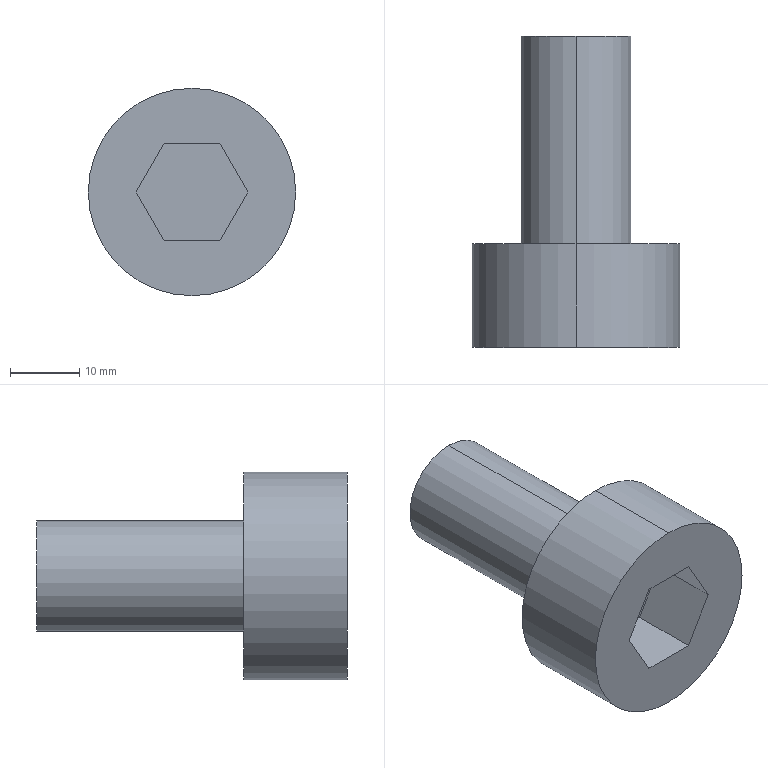Part | STEP file | M16X1.5 screw | 1 solid | 14 faces | box 30 x 45 x 30 mm | volume 14937 mm3 | plane 10 | cylinder 4 | commonest cylinder face diameters 16 x2 30 x2
STEP:
#1=CARTESIAN_POINT('',(0.,0.,0.));
#2=DIRECTION('',(0.,0.,1.));
#3=DIRECTION('',(1.,0.,0.));
#4=AXIS2_PLACEMENT_3D('',#1,#2,#3);
#5=CARTESIAN_POINT('',(0.,45.,-8.));
#6=VERTEX_POINT('',#5);
#7=CARTESIAN_POINT('',(0.,45.,8.));
#8=VERTEX_POINT('',#7);
#9=CARTESIAN_POINT('',(0.,45.,0.));
#10=DIRECTION('',(0.,-1.,0.));
#11=DIRECTION('',(0.,0.,-1.));
#12=AXIS2_PLACEMENT_3D('',#9,#10,#11);
#13=CIRCLE('',#12,8.);
#14=CARTESIAN_POINT('',(0.,0.,0.));
#15=DIRECTION('',(0.,-1.,0.));
#16=DIRECTION('',(0.,0.,-1.));
#17=AXIS2_PLACEMENT_3D('',#14,#15,#16);
#18=CYLINDRICAL_SURFACE('',#17,8.);
#19=CARTESIAN_POINT('',(0.,-45.));
#20=DIRECTION('',(1.,0.));
#21=VECTOR('',#20,1.);
#22=LINE('',#19,#21);
#23=(GEOMETRIC_REPRESENTATION_CONTEXT(2)PARAMETRIC_REPRESENTATION_CONTEXT()REPRESENTATION_CONTEXT('',''));
#24=DEFINITIONAL_REPRESENTATION('',(#22),#23);
#25=PCURVE('',#18,#24);
#26=CARTESIAN_POINT('',(8.,45.,0.));
#27=DIRECTION('',(0.,1.,0.));
#28=DIRECTION('',(0.,0.,1.));
#29=AXIS2_PLACEMENT_3D('',#26,#27,#28);
#30=PLANE('',#29);
#31=CARTESIAN_POINT('',(-8.,-8.));
#32=CARTESIAN_POINT('',(-8.,5.856));
#33=CARTESIAN_POINT('',(4.,-1.072));
#34=CARTESIAN_POINT('',(16.,-8.));
#35=CARTESIAN_POINT('',(4.,-14.928));
#36=CARTESIAN_POINT('',(-8.,-21.856));
#37=CARTESIAN_POINT('',(-8.,-8.));
#38=(BOUNDED_CURVE()B_SPLINE_CURVE(2,(#31,#32,#33,#34,#35,#36,#37),.UNSPECIFIED.,.T.,.F.)B_SPLINE_CURVE_WITH_KNOTS((1,2,2,2,2,1),(-2.094,0.,2.094,4.189,6.283,8.378),.UNSPECIFIED.)CURVE()GEOMETRIC_REPRESENTATION_ITEM()RATIONAL_B_SPLINE_CURVE((1.,0.5,1.,0.5,1.,0.5,1.))REPRESENTATION_ITEM(''));
#39=(GEOMETRIC_REPRESENTATION_CONTEXT(2)PARAMETRIC_REPRESENTATION_CONTEXT()REPRESENTATION_CONTEXT('',''));
#40=DEFINITIONAL_REPRESENTATION('',(#38),#39);
#41=PCURVE('',#30,#40);
#42=SURFACE_CURVE('',#13,(#25,#41),.PCURVE_S1.);
#43=EDGE_CURVE('',#6,#8,#42,.T.);
#44=ORIENTED_EDGE('',*,*,#43,.T.);
#45=CARTESIAN_POINT('',(0.,15.,8.));
#46=VERTEX_POINT('',#45);
#47=CARTESIAN_POINT('',(0.,0.,8.));
#48=DIRECTION('',(0.,-1.,0.));
#49=VECTOR('',#48,1.);
#50=LINE('',#47,#49);
#51=CARTESIAN_POINT('',(3.142,0.));
#52=DIRECTION('',(0.,1.));
#53=VECTOR('',#52,1.);
#54=LINE('',#51,#53);
#55=(GEOMETRIC_REPRESENTATION_CONTEXT(2)PARAMETRIC_REPRESENTATION_CONTEXT()REPRESENTATION_CONTEXT('',''));
#56=DEFINITIONAL_REPRESENTATION('',(#54),#55);
#57=PCURVE('',#18,#56);
#58=CARTESIAN_POINT('',(0.,0.,0.));
#59=DIRECTION('',(0.,-1.,0.));
#60=DIRECTION('',(0.,0.,-1.));
#61=AXIS2_PLACEMENT_3D('',#58,#59,#60);
#62=CYLINDRICAL_SURFACE('',#61,8.);
#63=CARTESIAN_POINT('',(3.142,0.));
#64=DIRECTION('',(0.,1.));
#65=VECTOR('',#64,1.);
#66=LINE('',#63,#65);
#67=(GEOMETRIC_REPRESENTATION_CONTEXT(2)PARAMETRIC_REPRESENTATION_CONTEXT()REPRESENTATION_CONTEXT('',''));
#68=DEFINITIONAL_REPRESENTATION('',(#66),#67);
#69=PCURVE('',#62,#68);
#70=SURFACE_CURVE('',#50,(#57,#69),.PCURVE_S1.);
#71=EDGE_CURVE('',#8,#46,#70,.T.);
#72=ORIENTED_EDGE('',*,*,#71,.T.);
#73=CARTESIAN_POINT('',(0.,15.,-8.));
#74=VERTEX_POINT('',#73);
#75=CARTESIAN_POINT('',(0.,15.,0.));
#76=DIRECTION('',(0.,-1.,0.));
#77=DIRECTION('',(0.,0.,-1.));
#78=AXIS2_PLACEMENT_3D('',#75,#76,#77);
#79=CIRCLE('',#78,8.);
#80=CARTESIAN_POINT('',(0.,-15.));
#81=DIRECTION('',(1.,0.));
#82=VECTOR('',#81,1.);
#83=LINE('',#80,#82);
#84=(GEOMETRIC_REPRESENTATION_CONTEXT(2)PARAMETRIC_REPRESENTATION_CONTEXT()REPRESENTATION_CONTEXT('',''));
#85=DEFINITIONAL_REPRESENTATION('',(#83),#84);
#86=PCURVE('',#18,#85);
#87=CARTESIAN_POINT('',(15.,15.,0.));
#88=DIRECTION('',(0.,1.,0.));
#89=DIRECTION('',(0.,0.,1.));
#90=AXIS2_PLACEMENT_3D('',#87,#88,#89);
#91=PLANE('',#90);
#92=CARTESIAN_POINT('',(-8.,-15.));
#93=CARTESIAN_POINT('',(-8.,-1.144));
#94=CARTESIAN_POINT('',(4.,-8.072));
#95=CARTESIAN_POINT('',(16.,-15.));
#96=CARTESIAN_POINT('',(4.,-21.928));
#97=CARTESIAN_POINT('',(-8.,-28.856));
#98=CARTESIAN_POINT('',(-8.,-15.));
#99=(BOUNDED_CURVE()B_SPLINE_CURVE(2,(#92,#93,#94,#95,#96,#97,#98),.UNSPECIFIED.,.T.,.F.)B_SPLINE_CURVE_WITH_KNOTS((1,2,2,2,2,1),(-2.094,0.,2.094,4.189,6.283,8.378),.UNSPECIFIED.)CURVE()GEOMETRIC_REPRESENTATION_ITEM()RATIONAL_B_SPLINE_CURVE((1.,0.5,1.,0.5,1.,0.5,1.))REPRESENTATION_ITEM(''));
#100=(GEOMETRIC_REPRESENTATION_CONTEXT(2)PARAMETRIC_REPRESENTATION_CONTEXT()REPRESENTATION_CONTEXT('',''));
#101=DEFINITIONAL_REPRESENTATION('',(#99),#100);
#102=PCURVE('',#91,#101);
#103=SURFACE_CURVE('',#79,(#86,#102),.PCURVE_S1.);
#104=EDGE_CURVE('',#74,#46,#103,.T.);
#105=ORIENTED_EDGE('',*,*,#104,.F.);
#106=CARTESIAN_POINT('',(0.,0.,-8.));
#107=DIRECTION('',(0.,-1.,0.));
#108=VECTOR('',#107,1.);
#109=LINE('',#106,#108);
#110=CARTESIAN_POINT('',(0.,0.));
#111=DIRECTION('',(0.,1.));
#112=VECTOR('',#111,1.);
#113=LINE('',#110,#112);
#114=(GEOMETRIC_REPRESENTATION_CONTEXT(2)PARAMETRIC_REPRESENTATION_CONTEXT()REPRESENTATION_CONTEXT('',''));
#115=DEFINITIONAL_REPRESENTATION('',(#113),#114);
#116=PCURVE('',#18,#115);
#117=CARTESIAN_POINT('',(6.283,0.));
#118=DIRECTION('',(0.,1.));
#119=VECTOR('',#118,1.);
#120=LINE('',#117,#119);
#121=(GEOMETRIC_REPRESENTATION_CONTEXT(2)PARAMETRIC_REPRESENTATION_CONTEXT()REPRESENTATION_CONTEXT('',''));
#122=DEFINITIONAL_REPRESENTATION('',(#120),#121);
#123=PCURVE('',#62,#122);
#124=SURFACE_CURVE('',#109,(#116,#123),.PCURVE_S1.);
#125=EDGE_CURVE('',#6,#74,#124,.T.);
#126=ORIENTED_EDGE('',*,*,#125,.F.);
#127=EDGE_LOOP('',(#44,#72,#105,#126));
#128=FACE_BOUND('',#127,.T.);
#129=ADVANCED_FACE('',(#128),#18,.T.);
#130=CARTESIAN_POINT('',(0.,15.,-15.));
#131=VERTEX_POINT('',#130);
#132=CARTESIAN_POINT('',(0.,15.,15.));
#133=VERTEX_POINT('',#132);
#134=CARTESIAN_POINT('',(0.,15.,0.));
#135=DIRECTION('',(0.,-1.,0.));
#136=DIRECTION('',(0.,0.,-1.));
#137=AXIS2_PLACEMENT_3D('',#134,#135,#136);
#138=CIRCLE('',#137,15.);
#139=CARTESIAN_POINT('',(0.,0.,0.));
#140=DIRECTION('',(0.,-1.,0.));
#141=DIRECTION('',(0.,0.,-1.));
#142=AXIS2_PLACEMENT_3D('',#139,#140,#141);
#143=CYLINDRICAL_SURFACE('',#142,15.);
#144=CARTESIAN_POINT('',(0.,-15.));
#145=DIRECTION('',(1.,0.));
#146=VECTOR('',#145,1.);
#147=LINE('',#144,#146);
#148=(GEOMETRIC_REPRESENTATION_CONTEXT(2)PARAMETRIC_REPRESENTATION_CONTEXT()REPRESENTATION_CONTEXT('',''));
#149=DEFINITIONAL_REPRESENTATION('',(#147),#148);
#150=PCURVE('',#143,#149);
#151=CARTESIAN_POINT('',(-15.,-15.));
#152=CARTESIAN_POINT('',(-15.,10.981));
#153=CARTESIAN_POINT('',(7.5,-2.01));
#154=CARTESIAN_POINT('',(30.,-15.));
#155=CARTESIAN_POINT('',(7.5,-27.99));
#156=CARTESIAN_POINT('',(-15.,-40.981));
#157=CARTESIAN_POINT('',(-15.,-15.));
#158=(BOUNDED_CURVE()B_SPLINE_CURVE(2,(#151,#152,#153,#154,#155,#156,#157),.UNSPECIFIED.,.T.,.F.)B_SPLINE_CURVE_WITH_KNOTS((1,2,2,2,2,1),(-2.094,0.,2.094,4.189,6.283,8.378),.UNSPECIFIED.)CURVE()GEOMETRIC_REPRESENTATION_ITEM()RATIONAL_B_SPLINE_CURVE((1.,0.5,1.,0.5,1.,0.5,1.))REPRESENTATION_ITEM(''));
#159=(GEOMETRIC_REPRESENTATION_CONTEXT(2)PARAMETRIC_REPRESENTATION_CONTEXT()REPRESENTATION_CONTEXT('',''));
#160=DEFINITIONAL_REPRESENTATION('',(#158),#159);
#161=PCURVE('',#91,#160);
#162=SURFACE_CURVE('',#138,(#150,#161),.PCURVE_S1.);
#163=EDGE_CURVE('',#131,#133,#162,.T.);
#164=ORIENTED_EDGE('',*,*,#163,.T.);
#165=CARTESIAN_POINT('',(0.,0.,15.));
#166=VERTEX_POINT('',#165);
#167=CARTESIAN_POINT('',(0.,0.,15.));
#168=DIRECTION('',(0.,-1.,0.));
#169=VECTOR('',#168,1.);
#170=LINE('',#167,#169);
#171=CARTESIAN_POINT('',(3.142,0.));
#172=DIRECTION('',(0.,1.));
#173=VECTOR('',#172,1.);
#174=LINE('',#171,#173);
#175=(GEOMETRIC_REPRESENTATION_CONTEXT(2)PARAMETRIC_REPRESENTATION_CONTEXT()REPRESENTATION_CONTEXT('',''));
#176=DEFINITIONAL_REPRESENTATION('',(#174),#175);
#177=PCURVE('',#143,#176);
#178=CARTESIAN_POINT('',(0.,0.,0.));
#179=DIRECTION('',(0.,-1.,0.));
#180=DIRECTION('',(0.,0.,-1.));
#181=AXIS2_PLACEMENT_3D('',#178,#179,#180);
#182=CYLINDRICAL_SURFACE('',#181,15.);
#183=CARTESIAN_POINT('',(3.142,0.));
#184=DIRECTION('',(0.,1.));
#185=VECTOR('',#184,1.);
#186=LINE('',#183,#185);
#187=(GEOMETRIC_REPRESENTATION_CONTEXT(2)PARAMETRIC_REPRESENTATION_CONTEXT()REPRESENTATION_CONTEXT('',''));
#188=DEFINITIONAL_REPRESENTATION('',(#186),#187);
#189=PCURVE('',#182,#188);
#190=SURFACE_CURVE('',#170,(#177,#189),.PCURVE_S1.);
#191=EDGE_CURVE('',#133,#166,#190,.T.);
#192=ORIENTED_EDGE('',*,*,#191,.T.);
#193=CARTESIAN_POINT('',(0.,0.,-15.));
#194=VERTEX_POINT('',#193);
#195=CARTESIAN_POINT('',(0.,0.,0.));
#196=DIRECTION('',(0.,-1.,0.));
#197=DIRECTION('',(0.,0.,-1.));
#198=AXIS2_PLACEMENT_3D('',#195,#196,#197);
#199=CIRCLE('',#198,15.);
#200=CARTESIAN_POINT('',(0.,0.));
#201=DIRECTION('',(1.,0.));
#202=VECTOR('',#201,1.);
#203=LINE('',#200,#202);
#204=(GEOMETRIC_REPRESENTATION_CONTEXT(2)PARAMETRIC_REPRESENTATION_CONTEXT()REPRESENTATION_CONTEXT('',''));
#205=DEFINITIONAL_REPRESENTATION('',(#203),#204);
#206=PCURVE('',#143,#205);
#207=CARTESIAN_POINT('',(0.,0.,0.));
#208=DIRECTION('',(0.,-1.,0.));
#209=DIRECTION('',(0.,0.,-1.));
#210=AXIS2_PLACEMENT_3D('',#207,#208,#209);
#211=PLANE('',#210);
#212=CARTESIAN_POINT('',(0.,0.));
#213=DIRECTION('',(1.,0.));
#214=AXIS2_PLACEMENT_2D('',#212,#213);
#215=CIRCLE('',#214,15.);
#216=(GEOMETRIC_REPRESENTATION_CONTEXT(2)PARAMETRIC_REPRESENTATION_CONTEXT()REPRESENTATION_CONTEXT('',''));
#217=DEFINITIONAL_REPRESENTATION('',(#215),#216);
#218=PCURVE('',#211,#217);
#219=SURFACE_CURVE('',#199,(#206,#218),.PCURVE_S1.);
#220=EDGE_CURVE('',#194,#166,#219,.T.);
#221=ORIENTED_EDGE('',*,*,#220,.F.);
#222=CARTESIAN_POINT('',(0.,0.,-15.));
#223=DIRECTION('',(0.,-1.,0.));
#224=VECTOR('',#223,1.);
#225=LINE('',#222,#224);
#226=CARTESIAN_POINT('',(0.,0.));
#227=DIRECTION('',(0.,1.));
#228=VECTOR('',#227,1.);
#229=LINE('',#226,#228);
#230=(GEOMETRIC_REPRESENTATION_CONTEXT(2)PARAMETRIC_REPRESENTATION_CONTEXT()REPRESENTATION_CONTEXT('',''));
#231=DEFINITIONAL_REPRESENTATION('',(#229),#230);
#232=PCURVE('',#143,#231);
#233=CARTESIAN_POINT('',(6.283,0.));
#234=DIRECTION('',(0.,1.));
#235=VECTOR('',#234,1.);
#236=LINE('',#233,#235);
#237=(GEOMETRIC_REPRESENTATION_CONTEXT(2)PARAMETRIC_REPRESENTATION_CONTEXT()REPRESENTATION_CONTEXT('',''));
#238=DEFINITIONAL_REPRESENTATION('',(#236),#237);
#239=PCURVE('',#182,#238);
#240=SURFACE_CURVE('',#225,(#232,#239),.PCURVE_S1.);
#241=EDGE_CURVE('',#131,#194,#240,.T.);
#242=ORIENTED_EDGE('',*,*,#241,.F.);
#243=EDGE_LOOP('',(#164,#192,#221,#242));
#244=FACE_BOUND('',#243,.T.);
#245=ADVANCED_FACE('',(#244),#143,.T.);
#246=CARTESIAN_POINT('',(-4.041,0.,7.));
#247=VERTEX_POINT('',#246);
#248=CARTESIAN_POINT('',(-8.083,0.,0.));
#249=VERTEX_POINT('',#248);
#250=CARTESIAN_POINT('',(-4.041,0.,7.));
#251=DIRECTION('',(-0.5,0.,-0.866));
#252=VECTOR('',#251,1.);
#253=LINE('',#250,#252);
#254=CARTESIAN_POINT('',(-7.,-4.041));
#255=DIRECTION('',(0.866,-0.5));
#256=VECTOR('',#255,1.);
#257=LINE('',#254,#256);
#258=(GEOMETRIC_REPRESENTATION_CONTEXT(2)PARAMETRIC_REPRESENTATION_CONTEXT()REPRESENTATION_CONTEXT('',''));
#259=DEFINITIONAL_REPRESENTATION('',(#257),#258);
#260=PCURVE('',#211,#259);
#261=CARTESIAN_POINT('',(-4.041,10.,7.));
#262=DIRECTION('',(-0.866,0.,0.5));
#263=DIRECTION('',(0.5,0.,0.866));
#264=AXIS2_PLACEMENT_3D('',#261,#262,#263);
#265=PLANE('',#264);
#266=CARTESIAN_POINT('',(0.,-10.));
#267=DIRECTION('',(-1.,0.));
#268=VECTOR('',#267,1.);
#269=LINE('',#266,#268);
#270=(GEOMETRIC_REPRESENTATION_CONTEXT(2)PARAMETRIC_REPRESENTATION_CONTEXT()REPRESENTATION_CONTEXT('',''));
#271=DEFINITIONAL_REPRESENTATION('',(#269),#270);
#272=PCURVE('',#265,#271);
#273=SURFACE_CURVE('',#253,(#260,#272),.PCURVE_S1.);
#274=EDGE_CURVE('',#247,#249,#273,.T.);
#275=ORIENTED_EDGE('',*,*,#274,.F.);
#276=CARTESIAN_POINT('',(4.041,0.,7.));
#277=VERTEX_POINT('',#276);
#278=CARTESIAN_POINT('',(4.041,0.,7.));
#279=DIRECTION('',(-1.,0.,0.));
#280=VECTOR('',#279,1.);
#281=LINE('',#278,#280);
#282=CARTESIAN_POINT('',(-7.,4.041));
#283=DIRECTION('',(0.,-1.));
#284=VECTOR('',#283,1.);
#285=LINE('',#282,#284);
#286=(GEOMETRIC_REPRESENTATION_CONTEXT(2)PARAMETRIC_REPRESENTATION_CONTEXT()REPRESENTATION_CONTEXT('',''));
#287=DEFINITIONAL_REPRESENTATION('',(#285),#286);
#288=PCURVE('',#211,#287);
#289=CARTESIAN_POINT('',(4.041,10.,7.));
#290=DIRECTION('',(0.,0.,1.));
#291=DIRECTION('',(1.,0.,0.));
#292=AXIS2_PLACEMENT_3D('',#289,#290,#291);
#293=PLANE('',#292);
#294=CARTESIAN_POINT('',(0.,-10.));
#295=DIRECTION('',(-1.,0.));
#296=VECTOR('',#295,1.);
#297=LINE('',#294,#296);
#298=(GEOMETRIC_REPRESENTATION_CONTEXT(2)PARAMETRIC_REPRESENTATION_CONTEXT()REPRESENTATION_CONTEXT('',''));
#299=DEFINITIONAL_REPRESENTATION('',(#297),#298);
#300=PCURVE('',#293,#299);
#301=SURFACE_CURVE('',#281,(#288,#300),.PCURVE_S1.);
#302=EDGE_CURVE('',#277,#247,#301,.T.);
#303=ORIENTED_EDGE('',*,*,#302,.F.);
#304=CARTESIAN_POINT('',(8.083,0.,0.));
#305=VERTEX_POINT('',#304);
#306=CARTESIAN_POINT('',(8.083,0.,0.));
#307=DIRECTION('',(-0.5,0.,0.866));
#308=VECTOR('',#307,1.);
#309=LINE('',#306,#308);
#310=CARTESIAN_POINT('',(0.,8.083));
#311=DIRECTION('',(-0.866,-0.5));
#312=VECTOR('',#311,1.);
#313=LINE('',#310,#312);
#314=(GEOMETRIC_REPRESENTATION_CONTEXT(2)PARAMETRIC_REPRESENTATION_CONTEXT()REPRESENTATION_CONTEXT('',''));
#315=DEFINITIONAL_REPRESENTATION('',(#313),#314);
#316=PCURVE('',#211,#315);
#317=CARTESIAN_POINT('',(8.083,10.,0.));
#318=DIRECTION('',(0.866,0.,0.5));
#319=DIRECTION('',(0.5,0.,-0.866));
#320=AXIS2_PLACEMENT_3D('',#317,#318,#319);
#321=PLANE('',#320);
#322=CARTESIAN_POINT('',(0.,-10.));
#323=DIRECTION('',(-1.,0.));
#324=VECTOR('',#323,1.);
#325=LINE('',#322,#324);
#326=(GEOMETRIC_REPRESENTATION_CONTEXT(2)PARAMETRIC_REPRESENTATION_CONTEXT()REPRESENTATION_CONTEXT('',''));
#327=DEFINITIONAL_REPRESENTATION('',(#325),#326);
#328=PCURVE('',#321,#327);
#329=SURFACE_CURVE('',#309,(#316,#328),.PCURVE_S1.);
#330=EDGE_CURVE('',#305,#277,#329,.T.);
#331=ORIENTED_EDGE('',*,*,#330,.F.);
#332=CARTESIAN_POINT('',(4.041,0.,-7.));
#333=VERTEX_POINT('',#332);
#334=CARTESIAN_POINT('',(4.041,0.,-7.));
#335=DIRECTION('',(0.5,0.,0.866));
#336=VECTOR('',#335,1.);
#337=LINE('',#334,#336);
#338=CARTESIAN_POINT('',(7.,4.041));
#339=DIRECTION('',(-0.866,0.5));
#340=VECTOR('',#339,1.);
#341=LINE('',#338,#340);
#342=(GEOMETRIC_REPRESENTATION_CONTEXT(2)PARAMETRIC_REPRESENTATION_CONTEXT()REPRESENTATION_CONTEXT('',''));
#343=DEFINITIONAL_REPRESENTATION('',(#341),#342);
#344=PCURVE('',#211,#343);
#345=CARTESIAN_POINT('',(4.041,10.,-7.));
#346=DIRECTION('',(0.866,0.,-0.5));
#347=DIRECTION('',(-0.5,0.,-0.866));
#348=AXIS2_PLACEMENT_3D('',#345,#346,#347);
#349=PLANE('',#348);
#350=CARTESIAN_POINT('',(0.,-10.));
#351=DIRECTION('',(-1.,0.));
#352=VECTOR('',#351,1.);
#353=LINE('',#350,#352);
#354=(GEOMETRIC_REPRESENTATION_CONTEXT(2)PARAMETRIC_REPRESENTATION_CONTEXT()REPRESENTATION_CONTEXT('',''));
#355=DEFINITIONAL_REPRESENTATION('',(#353),#354);
#356=PCURVE('',#349,#355);
#357=SURFACE_CURVE('',#337,(#344,#356),.PCURVE_S1.);
#358=EDGE_CURVE('',#333,#305,#357,.T.);
#359=ORIENTED_EDGE('',*,*,#358,.F.);
#360=CARTESIAN_POINT('',(-4.041,0.,-7.));
#361=VERTEX_POINT('',#360);
#362=CARTESIAN_POINT('',(-4.041,0.,-7.));
#363=DIRECTION('',(1.,0.,0.));
#364=VECTOR('',#363,1.);
#365=LINE('',#362,#364);
#366=CARTESIAN_POINT('',(7.,-4.041));
#367=DIRECTION('',(0.,1.));
#368=VECTOR('',#367,1.);
#369=LINE('',#366,#368);
#370=(GEOMETRIC_REPRESENTATION_CONTEXT(2)PARAMETRIC_REPRESENTATION_CONTEXT()REPRESENTATION_CONTEXT('',''));
#371=DEFINITIONAL_REPRESENTATION('',(#369),#370);
#372=PCURVE('',#211,#371);
#373=CARTESIAN_POINT('',(-4.041,10.,-7.));
#374=DIRECTION('',(0.,0.,-1.));
#375=DIRECTION('',(-1.,0.,0.));
#376=AXIS2_PLACEMENT_3D('',#373,#374,#375);
#377=PLANE('',#376);
#378=CARTESIAN_POINT('',(0.,-10.));
#379=DIRECTION('',(-1.,0.));
#380=VECTOR('',#379,1.);
#381=LINE('',#378,#380);
#382=(GEOMETRIC_REPRESENTATION_CONTEXT(2)PARAMETRIC_REPRESENTATION_CONTEXT()REPRESENTATION_CONTEXT('',''));
#383=DEFINITIONAL_REPRESENTATION('',(#381),#382);
#384=PCURVE('',#377,#383);
#385=SURFACE_CURVE('',#365,(#372,#384),.PCURVE_S1.);
#386=EDGE_CURVE('',#361,#333,#385,.T.);
#387=ORIENTED_EDGE('',*,*,#386,.F.);
#388=CARTESIAN_POINT('',(-8.083,0.,0.));
#389=DIRECTION('',(0.5,0.,-0.866));
#390=VECTOR('',#389,1.);
#391=LINE('',#388,#390);
#392=CARTESIAN_POINT('',(0.,-8.083));
#393=DIRECTION('',(0.866,0.5));
#394=VECTOR('',#393,1.);
#395=LINE('',#392,#394);
#396=(GEOMETRIC_REPRESENTATION_CONTEXT(2)PARAMETRIC_REPRESENTATION_CONTEXT()REPRESENTATION_CONTEXT('',''));
#397=DEFINITIONAL_REPRESENTATION('',(#395),#396);
#398=PCURVE('',#211,#397);
#399=CARTESIAN_POINT('',(-8.083,10.,0.));
#400=DIRECTION('',(-0.866,0.,-0.5));
#401=DIRECTION('',(-0.5,0.,0.866));
#402=AXIS2_PLACEMENT_3D('',#399,#400,#401);
#403=PLANE('',#402);
#404=CARTESIAN_POINT('',(0.,-10.));
#405=DIRECTION('',(-1.,0.));
#406=VECTOR('',#405,1.);
#407=LINE('',#404,#406);
#408=(GEOMETRIC_REPRESENTATION_CONTEXT(2)PARAMETRIC_REPRESENTATION_CONTEXT()REPRESENTATION_CONTEXT('',''));
#409=DEFINITIONAL_REPRESENTATION('',(#407),#408);
#410=PCURVE('',#403,#409);
#411=SURFACE_CURVE('',#391,(#398,#410),.PCURVE_S1.);
#412=EDGE_CURVE('',#249,#361,#411,.T.);
#413=ORIENTED_EDGE('',*,*,#412,.F.);
#414=EDGE_LOOP('',(#275,#303,#331,#359,#387,#413));
#415=FACE_BOUND('',#414,.T.);
#416=ORIENTED_EDGE('',*,*,#220,.T.);
#417=CARTESIAN_POINT('',(0.,0.,0.));
#418=DIRECTION('',(0.,-1.,0.));
#419=DIRECTION('',(0.,0.,-1.));
#420=AXIS2_PLACEMENT_3D('',#417,#418,#419);
#421=CIRCLE('',#420,15.);
#422=CARTESIAN_POINT('',(0.,0.));
#423=DIRECTION('',(1.,0.));
#424=AXIS2_PLACEMENT_2D('',#422,#423);
#425=CIRCLE('',#424,15.);
#426=(GEOMETRIC_REPRESENTATION_CONTEXT(2)PARAMETRIC_REPRESENTATION_CONTEXT()REPRESENTATION_CONTEXT('',''));
#427=DEFINITIONAL_REPRESENTATION('',(#425),#426);
#428=PCURVE('',#211,#427);
#429=CARTESIAN_POINT('',(0.,0.));
#430=DIRECTION('',(1.,0.));
#431=VECTOR('',#430,1.);
#432=LINE('',#429,#431);
#433=(GEOMETRIC_REPRESENTATION_CONTEXT(2)PARAMETRIC_REPRESENTATION_CONTEXT()REPRESENTATION_CONTEXT('',''));
#434=DEFINITIONAL_REPRESENTATION('',(#432),#433);
#435=PCURVE('',#182,#434);
#436=SURFACE_CURVE('',#421,(#428,#435),.PCURVE_S1.);
#437=EDGE_CURVE('',#166,#194,#436,.T.);
#438=ORIENTED_EDGE('',*,*,#437,.T.);
#439=EDGE_LOOP('',(#416,#438));
#440=FACE_BOUND('',#439,.T.);
#441=ADVANCED_FACE('',(#415,#440),#211,.T.);
#442=ORIENTED_EDGE('',*,*,#191,.F.);
#443=CARTESIAN_POINT('',(0.,15.,0.));
#444=DIRECTION('',(0.,-1.,0.));
#445=DIRECTION('',(0.,0.,-1.));
#446=AXIS2_PLACEMENT_3D('',#443,#444,#445);
#447=CIRCLE('',#446,15.);
#448=CARTESIAN_POINT('',(0.,-15.));
#449=DIRECTION('',(1.,0.));
#450=VECTOR('',#449,1.);
#451=LINE('',#448,#450);
#452=(GEOMETRIC_REPRESENTATION_CONTEXT(2)PARAMETRIC_REPRESENTATION_CONTEXT()REPRESENTATION_CONTEXT('',''));
#453=DEFINITIONAL_REPRESENTATION('',(#451),#452);
#454=PCURVE('',#182,#453);
#455=CARTESIAN_POINT('',(-15.,-15.));
#456=CARTESIAN_POINT('',(-15.,10.981));
#457=CARTESIAN_POINT('',(7.5,-2.01));
#458=CARTESIAN_POINT('',(30.,-15.));
#459=CARTESIAN_POINT('',(7.5,-27.99));
#460=CARTESIAN_POINT('',(-15.,-40.981));
#461=CARTESIAN_POINT('',(-15.,-15.));
#462=(BOUNDED_CURVE()B_SPLINE_CURVE(2,(#455,#456,#457,#458,#459,#460,#461),.UNSPECIFIED.,.T.,.F.)B_SPLINE_CURVE_WITH_KNOTS((1,2,2,2,2,1),(-2.094,0.,2.094,4.189,6.283,8.378),.UNSPECIFIED.)CURVE()GEOMETRIC_REPRESENTATION_ITEM()RATIONAL_B_SPLINE_CURVE((1.,0.5,1.,0.5,1.,0.5,1.))REPRESENTATION_ITEM(''));
#463=(GEOMETRIC_REPRESENTATION_CONTEXT(2)PARAMETRIC_REPRESENTATION_CONTEXT()REPRESENTATION_CONTEXT('',''));
#464=DEFINITIONAL_REPRESENTATION('',(#462),#463);
#465=PCURVE('',#91,#464);
#466=SURFACE_CURVE('',#447,(#454,#465),.PCURVE_S1.);
#467=EDGE_CURVE('',#133,#131,#466,.T.);
#468=ORIENTED_EDGE('',*,*,#467,.T.);
#469=ORIENTED_EDGE('',*,*,#241,.T.);
#470=ORIENTED_EDGE('',*,*,#437,.F.);
#471=EDGE_LOOP('',(#442,#468,#469,#470));
#472=FACE_BOUND('',#471,.T.);
#473=ADVANCED_FACE('',(#472),#182,.T.);
#474=ORIENTED_EDGE('',*,*,#104,.T.);
#475=CARTESIAN_POINT('',(0.,15.,0.));
#476=DIRECTION('',(0.,-1.,0.));
#477=DIRECTION('',(0.,0.,-1.));
#478=AXIS2_PLACEMENT_3D('',#475,#476,#477);
#479=CIRCLE('',#478,8.);
#480=CARTESIAN_POINT('',(-8.,-15.));
#481=CARTESIAN_POINT('',(-8.,-1.144));
#482=CARTESIAN_POINT('',(4.,-8.072));
#483=CARTESIAN_POINT('',(16.,-15.));
#484=CARTESIAN_POINT('',(4.,-21.928));
#485=CARTESIAN_POINT('',(-8.,-28.856));
#486=CARTESIAN_POINT('',(-8.,-15.));
#487=(BOUNDED_CURVE()B_SPLINE_CURVE(2,(#480,#481,#482,#483,#484,#485,#486),.UNSPECIFIED.,.T.,.F.)B_SPLINE_CURVE_WITH_KNOTS((1,2,2,2,2,1),(-2.094,0.,2.094,4.189,6.283,8.378),.UNSPECIFIED.)CURVE()GEOMETRIC_REPRESENTATION_ITEM()RATIONAL_B_SPLINE_CURVE((1.,0.5,1.,0.5,1.,0.5,1.))REPRESENTATION_ITEM(''));
#488=(GEOMETRIC_REPRESENTATION_CONTEXT(2)PARAMETRIC_REPRESENTATION_CONTEXT()REPRESENTATION_CONTEXT('',''));
#489=DEFINITIONAL_REPRESENTATION('',(#487),#488);
#490=PCURVE('',#91,#489);
#491=CARTESIAN_POINT('',(0.,-15.));
#492=DIRECTION('',(1.,0.));
#493=VECTOR('',#492,1.);
#494=LINE('',#491,#493);
#495=(GEOMETRIC_REPRESENTATION_CONTEXT(2)PARAMETRIC_REPRESENTATION_CONTEXT()REPRESENTATION_CONTEXT('',''));
#496=DEFINITIONAL_REPRESENTATION('',(#494),#495);
#497=PCURVE('',#62,#496);
#498=SURFACE_CURVE('',#479,(#490,#497),.PCURVE_S1.);
#499=EDGE_CURVE('',#46,#74,#498,.T.);
#500=ORIENTED_EDGE('',*,*,#499,.T.);
#501=EDGE_LOOP('',(#474,#500));
#502=FACE_BOUND('',#501,.T.);
#503=ORIENTED_EDGE('',*,*,#163,.F.);
#504=ORIENTED_EDGE('',*,*,#467,.F.);
#505=EDGE_LOOP('',(#503,#504));
#506=FACE_BOUND('',#505,.T.);
#507=ADVANCED_FACE('',(#502,#506),#91,.T.);
#508=ORIENTED_EDGE('',*,*,#71,.F.);
#509=CARTESIAN_POINT('',(0.,45.,0.));
#510=DIRECTION('',(0.,-1.,0.));
#511=DIRECTION('',(0.,0.,-1.));
#512=AXIS2_PLACEMENT_3D('',#509,#510,#511);
#513=CIRCLE('',#512,8.);
#514=CARTESIAN_POINT('',(0.,-45.));
#515=DIRECTION('',(1.,0.));
#516=VECTOR('',#515,1.);
#517=LINE('',#514,#516);
#518=(GEOMETRIC_REPRESENTATION_CONTEXT(2)PARAMETRIC_REPRESENTATION_CONTEXT()REPRESENTATION_CONTEXT('',''));
#519=DEFINITIONAL_REPRESENTATION('',(#517),#518);
#520=PCURVE('',#62,#519);
#521=CARTESIAN_POINT('',(-8.,-8.));
#522=CARTESIAN_POINT('',(-8.,5.856));
#523=CARTESIAN_POINT('',(4.,-1.072));
#524=CARTESIAN_POINT('',(16.,-8.));
#525=CARTESIAN_POINT('',(4.,-14.928));
#526=CARTESIAN_POINT('',(-8.,-21.856));
#527=CARTESIAN_POINT('',(-8.,-8.));
#528=(BOUNDED_CURVE()B_SPLINE_CURVE(2,(#521,#522,#523,#524,#525,#526,#527),.UNSPECIFIED.,.T.,.F.)B_SPLINE_CURVE_WITH_KNOTS((1,2,2,2,2,1),(-2.094,0.,2.094,4.189,6.283,8.378),.UNSPECIFIED.)CURVE()GEOMETRIC_REPRESENTATION_ITEM()RATIONAL_B_SPLINE_CURVE((1.,0.5,1.,0.5,1.,0.5,1.))REPRESENTATION_ITEM(''));
#529=(GEOMETRIC_REPRESENTATION_CONTEXT(2)PARAMETRIC_REPRESENTATION_CONTEXT()REPRESENTATION_CONTEXT('',''));
#530=DEFINITIONAL_REPRESENTATION('',(#528),#529);
#531=PCURVE('',#30,#530);
#532=SURFACE_CURVE('',#513,(#520,#531),.PCURVE_S1.);
#533=EDGE_CURVE('',#8,#6,#532,.T.);
#534=ORIENTED_EDGE('',*,*,#533,.T.);
#535=ORIENTED_EDGE('',*,*,#125,.T.);
#536=ORIENTED_EDGE('',*,*,#499,.F.);
#537=EDGE_LOOP('',(#508,#534,#535,#536));
#538=FACE_BOUND('',#537,.T.);
#539=ADVANCED_FACE('',(#538),#62,.T.);
#540=ORIENTED_EDGE('',*,*,#43,.F.);
#541=ORIENTED_EDGE('',*,*,#533,.F.);
#542=EDGE_LOOP('',(#540,#541));
#543=FACE_BOUND('',#542,.T.);
#544=ADVANCED_FACE('',(#543),#30,.T.);
#545=ORIENTED_EDGE('',*,*,#274,.T.);
#546=CARTESIAN_POINT('',(-8.083,10.,0.));
#547=VERTEX_POINT('',#546);
#548=CARTESIAN_POINT('',(-8.083,10.,0.));
#549=DIRECTION('',(0.,-1.,0.));
#550=VECTOR('',#549,1.);
#551=LINE('',#548,#550);
#552=CARTESIAN_POINT('',(-8.083,0.));
#553=DIRECTION('',(0.,-1.));
#554=VECTOR('',#553,1.);
#555=LINE('',#552,#554);
#556=(GEOMETRIC_REPRESENTATION_CONTEXT(2)PARAMETRIC_REPRESENTATION_CONTEXT()REPRESENTATION_CONTEXT('',''));
#557=DEFINITIONAL_REPRESENTATION('',(#555),#556);
#558=PCURVE('',#265,#557);
#559=CARTESIAN_POINT('',(0.,0.));
#560=DIRECTION('',(0.,-1.));
#561=VECTOR('',#560,1.);
#562=LINE('',#559,#561);
#563=(GEOMETRIC_REPRESENTATION_CONTEXT(2)PARAMETRIC_REPRESENTATION_CONTEXT()REPRESENTATION_CONTEXT('',''));
#564=DEFINITIONAL_REPRESENTATION('',(#562),#563);
#565=PCURVE('',#403,#564);
#566=SURFACE_CURVE('',#551,(#558,#565),.PCURVE_S1.);
#567=EDGE_CURVE('',#547,#249,#566,.T.);
#568=ORIENTED_EDGE('',*,*,#567,.F.);
#569=CARTESIAN_POINT('',(-4.041,10.,7.));
#570=VERTEX_POINT('',#569);
#571=CARTESIAN_POINT('',(-4.041,10.,7.));
#572=DIRECTION('',(-0.5,0.,-0.866));
#573=VECTOR('',#572,1.);
#574=LINE('',#571,#573);
#575=CARTESIAN_POINT('',(0.,0.));
#576=DIRECTION('',(-1.,0.));
#577=VECTOR('',#576,1.);
#578=LINE('',#575,#577);
#579=(GEOMETRIC_REPRESENTATION_CONTEXT(2)PARAMETRIC_REPRESENTATION_CONTEXT()REPRESENTATION_CONTEXT('',''));
#580=DEFINITIONAL_REPRESENTATION('',(#578),#579);
#581=PCURVE('',#265,#580);
#582=CARTESIAN_POINT('',(0.,10.,0.));
#583=DIRECTION('',(0.,-1.,0.));
#584=DIRECTION('',(0.,0.,-1.));
#585=AXIS2_PLACEMENT_3D('',#582,#583,#584);
#586=PLANE('',#585);
#587=CARTESIAN_POINT('',(-7.,-4.041));
#588=DIRECTION('',(0.866,-0.5));
#589=VECTOR('',#588,1.);
#590=LINE('',#587,#589);
#591=(GEOMETRIC_REPRESENTATION_CONTEXT(2)PARAMETRIC_REPRESENTATION_CONTEXT()REPRESENTATION_CONTEXT('',''));
#592=DEFINITIONAL_REPRESENTATION('',(#590),#591);
#593=PCURVE('',#586,#592);
#594=SURFACE_CURVE('',#574,(#581,#593),.PCURVE_S1.);
#595=EDGE_CURVE('',#570,#547,#594,.T.);
#596=ORIENTED_EDGE('',*,*,#595,.F.);
#597=CARTESIAN_POINT('',(-4.041,10.,7.));
#598=DIRECTION('',(0.,-1.,0.));
#599=VECTOR('',#598,1.);
#600=LINE('',#597,#599);
#601=CARTESIAN_POINT('',(0.,0.));
#602=DIRECTION('',(0.,-1.));
#603=VECTOR('',#602,1.);
#604=LINE('',#601,#603);
#605=(GEOMETRIC_REPRESENTATION_CONTEXT(2)PARAMETRIC_REPRESENTATION_CONTEXT()REPRESENTATION_CONTEXT('',''));
#606=DEFINITIONAL_REPRESENTATION('',(#604),#605);
#607=PCURVE('',#265,#606);
#608=CARTESIAN_POINT('',(-8.083,0.));
#609=DIRECTION('',(0.,-1.));
#610=VECTOR('',#609,1.);
#611=LINE('',#608,#610);
#612=(GEOMETRIC_REPRESENTATION_CONTEXT(2)PARAMETRIC_REPRESENTATION_CONTEXT()REPRESENTATION_CONTEXT('',''));
#613=DEFINITIONAL_REPRESENTATION('',(#611),#612);
#614=PCURVE('',#293,#613);
#615=SURFACE_CURVE('',#600,(#607,#614),.PCURVE_S1.);
#616=EDGE_CURVE('',#570,#247,#615,.T.);
#617=ORIENTED_EDGE('',*,*,#616,.T.);
#618=EDGE_LOOP('',(#545,#568,#596,#617));
#619=FACE_BOUND('',#618,.T.);
#620=ADVANCED_FACE('',(#619),#265,.F.);
#621=ORIENTED_EDGE('',*,*,#302,.T.);
#622=ORIENTED_EDGE('',*,*,#616,.F.);
#623=CARTESIAN_POINT('',(4.041,10.,7.));
#624=VERTEX_POINT('',#623);
#625=CARTESIAN_POINT('',(4.041,10.,7.));
#626=DIRECTION('',(-1.,0.,0.));
#627=VECTOR('',#626,1.);
#628=LINE('',#625,#627);
#629=CARTESIAN_POINT('',(0.,0.));
#630=DIRECTION('',(-1.,0.));
#631=VECTOR('',#630,1.);
#632=LINE('',#629,#631);
#633=(GEOMETRIC_REPRESENTATION_CONTEXT(2)PARAMETRIC_REPRESENTATION_CONTEXT()REPRESENTATION_CONTEXT('',''));
#634=DEFINITIONAL_REPRESENTATION('',(#632),#633);
#635=PCURVE('',#293,#634);
#636=CARTESIAN_POINT('',(-7.,4.041));
#637=DIRECTION('',(0.,-1.));
#638=VECTOR('',#637,1.);
#639=LINE('',#636,#638);
#640=(GEOMETRIC_REPRESENTATION_CONTEXT(2)PARAMETRIC_REPRESENTATION_CONTEXT()REPRESENTATION_CONTEXT('',''));
#641=DEFINITIONAL_REPRESENTATION('',(#639),#640);
#642=PCURVE('',#586,#641);
#643=SURFACE_CURVE('',#628,(#635,#642),.PCURVE_S1.);
#644=EDGE_CURVE('',#624,#570,#643,.T.);
#645=ORIENTED_EDGE('',*,*,#644,.F.);
#646=CARTESIAN_POINT('',(4.041,10.,7.));
#647=DIRECTION('',(0.,-1.,0.));
#648=VECTOR('',#647,1.);
#649=LINE('',#646,#648);
#650=CARTESIAN_POINT('',(0.,0.));
#651=DIRECTION('',(0.,-1.));
#652=VECTOR('',#651,1.);
#653=LINE('',#650,#652);
#654=(GEOMETRIC_REPRESENTATION_CONTEXT(2)PARAMETRIC_REPRESENTATION_CONTEXT()REPRESENTATION_CONTEXT('',''));
#655=DEFINITIONAL_REPRESENTATION('',(#653),#654);
#656=PCURVE('',#293,#655);
#657=CARTESIAN_POINT('',(-8.083,0.));
#658=DIRECTION('',(0.,-1.));
#659=VECTOR('',#658,1.);
#660=LINE('',#657,#659);
#661=(GEOMETRIC_REPRESENTATION_CONTEXT(2)PARAMETRIC_REPRESENTATION_CONTEXT()REPRESENTATION_CONTEXT('',''));
#662=DEFINITIONAL_REPRESENTATION('',(#660),#661);
#663=PCURVE('',#321,#662);
#664=SURFACE_CURVE('',#649,(#656,#663),.PCURVE_S1.);
#665=EDGE_CURVE('',#624,#277,#664,.T.);
#666=ORIENTED_EDGE('',*,*,#665,.T.);
#667=EDGE_LOOP('',(#621,#622,#645,#666));
#668=FACE_BOUND('',#667,.T.);
#669=ADVANCED_FACE('',(#668),#293,.F.);
#670=ORIENTED_EDGE('',*,*,#330,.T.);
#671=ORIENTED_EDGE('',*,*,#665,.F.);
#672=CARTESIAN_POINT('',(8.083,10.,0.));
#673=VERTEX_POINT('',#672);
#674=CARTESIAN_POINT('',(8.083,10.,0.));
#675=DIRECTION('',(-0.5,0.,0.866));
#676=VECTOR('',#675,1.);
#677=LINE('',#674,#676);
#678=CARTESIAN_POINT('',(0.,0.));
#679=DIRECTION('',(-1.,0.));
#680=VECTOR('',#679,1.);
#681=LINE('',#678,#680);
#682=(GEOMETRIC_REPRESENTATION_CONTEXT(2)PARAMETRIC_REPRESENTATION_CONTEXT()REPRESENTATION_CONTEXT('',''));
#683=DEFINITIONAL_REPRESENTATION('',(#681),#682);
#684=PCURVE('',#321,#683);
#685=CARTESIAN_POINT('',(0.,8.083));
#686=DIRECTION('',(-0.866,-0.5));
#687=VECTOR('',#686,1.);
#688=LINE('',#685,#687);
#689=(GEOMETRIC_REPRESENTATION_CONTEXT(2)PARAMETRIC_REPRESENTATION_CONTEXT()REPRESENTATION_CONTEXT('',''));
#690=DEFINITIONAL_REPRESENTATION('',(#688),#689);
#691=PCURVE('',#586,#690);
#692=SURFACE_CURVE('',#677,(#684,#691),.PCURVE_S1.);
#693=EDGE_CURVE('',#673,#624,#692,.T.);
#694=ORIENTED_EDGE('',*,*,#693,.F.);
#695=CARTESIAN_POINT('',(8.083,10.,0.));
#696=DIRECTION('',(0.,-1.,0.));
#697=VECTOR('',#696,1.);
#698=LINE('',#695,#697);
#699=CARTESIAN_POINT('',(0.,0.));
#700=DIRECTION('',(0.,-1.));
#701=VECTOR('',#700,1.);
#702=LINE('',#699,#701);
#703=(GEOMETRIC_REPRESENTATION_CONTEXT(2)PARAMETRIC_REPRESENTATION_CONTEXT()REPRESENTATION_CONTEXT('',''));
#704=DEFINITIONAL_REPRESENTATION('',(#702),#703);
#705=PCURVE('',#321,#704);
#706=CARTESIAN_POINT('',(-8.083,0.));
#707=DIRECTION('',(0.,-1.));
#708=VECTOR('',#707,1.);
#709=LINE('',#706,#708);
#710=(GEOMETRIC_REPRESENTATION_CONTEXT(2)PARAMETRIC_REPRESENTATION_CONTEXT()REPRESENTATION_CONTEXT('',''));
#711=DEFINITIONAL_REPRESENTATION('',(#709),#710);
#712=PCURVE('',#349,#711);
#713=SURFACE_CURVE('',#698,(#705,#712),.PCURVE_S1.);
#714=EDGE_CURVE('',#673,#305,#713,.T.);
#715=ORIENTED_EDGE('',*,*,#714,.T.);
#716=EDGE_LOOP('',(#670,#671,#694,#715));
#717=FACE_BOUND('',#716,.T.);
#718=ADVANCED_FACE('',(#717),#321,.F.);
#719=ORIENTED_EDGE('',*,*,#358,.T.);
#720=ORIENTED_EDGE('',*,*,#714,.F.);
#721=CARTESIAN_POINT('',(4.041,10.,-7.));
#722=VERTEX_POINT('',#721);
#723=CARTESIAN_POINT('',(4.041,10.,-7.));
#724=DIRECTION('',(0.5,0.,0.866));
#725=VECTOR('',#724,1.);
#726=LINE('',#723,#725);
#727=CARTESIAN_POINT('',(0.,0.));
#728=DIRECTION('',(-1.,0.));
#729=VECTOR('',#728,1.);
#730=LINE('',#727,#729);
#731=(GEOMETRIC_REPRESENTATION_CONTEXT(2)PARAMETRIC_REPRESENTATION_CONTEXT()REPRESENTATION_CONTEXT('',''));
#732=DEFINITIONAL_REPRESENTATION('',(#730),#731);
#733=PCURVE('',#349,#732);
#734=CARTESIAN_POINT('',(7.,4.041));
#735=DIRECTION('',(-0.866,0.5));
#736=VECTOR('',#735,1.);
#737=LINE('',#734,#736);
#738=(GEOMETRIC_REPRESENTATION_CONTEXT(2)PARAMETRIC_REPRESENTATION_CONTEXT()REPRESENTATION_CONTEXT('',''));
#739=DEFINITIONAL_REPRESENTATION('',(#737),#738);
#740=PCURVE('',#586,#739);
#741=SURFACE_CURVE('',#726,(#733,#740),.PCURVE_S1.);
#742=EDGE_CURVE('',#722,#673,#741,.T.);
#743=ORIENTED_EDGE('',*,*,#742,.F.);
#744=CARTESIAN_POINT('',(4.041,10.,-7.));
#745=DIRECTION('',(0.,-1.,0.));
#746=VECTOR('',#745,1.);
#747=LINE('',#744,#746);
#748=CARTESIAN_POINT('',(0.,0.));
#749=DIRECTION('',(0.,-1.));
#750=VECTOR('',#749,1.);
#751=LINE('',#748,#750);
#752=(GEOMETRIC_REPRESENTATION_CONTEXT(2)PARAMETRIC_REPRESENTATION_CONTEXT()REPRESENTATION_CONTEXT('',''));
#753=DEFINITIONAL_REPRESENTATION('',(#751),#752);
#754=PCURVE('',#349,#753);
#755=CARTESIAN_POINT('',(-8.083,0.));
#756=DIRECTION('',(0.,-1.));
#757=VECTOR('',#756,1.);
#758=LINE('',#755,#757);
#759=(GEOMETRIC_REPRESENTATION_CONTEXT(2)PARAMETRIC_REPRESENTATION_CONTEXT()REPRESENTATION_CONTEXT('',''));
#760=DEFINITIONAL_REPRESENTATION('',(#758),#759);
#761=PCURVE('',#377,#760);
#762=SURFACE_CURVE('',#747,(#754,#761),.PCURVE_S1.);
#763=EDGE_CURVE('',#722,#333,#762,.T.);
#764=ORIENTED_EDGE('',*,*,#763,.T.);
#765=EDGE_LOOP('',(#719,#720,#743,#764));
#766=FACE_BOUND('',#765,.T.);
#767=ADVANCED_FACE('',(#766),#349,.F.);
#768=ORIENTED_EDGE('',*,*,#386,.T.);
#769=ORIENTED_EDGE('',*,*,#763,.F.);
#770=CARTESIAN_POINT('',(-4.041,10.,-7.));
#771=VERTEX_POINT('',#770);
#772=CARTESIAN_POINT('',(-4.041,10.,-7.));
#773=DIRECTION('',(1.,0.,0.));
#774=VECTOR('',#773,1.);
#775=LINE('',#772,#774);
#776=CARTESIAN_POINT('',(0.,0.));
#777=DIRECTION('',(-1.,0.));
#778=VECTOR('',#777,1.);
#779=LINE('',#776,#778);
#780=(GEOMETRIC_REPRESENTATION_CONTEXT(2)PARAMETRIC_REPRESENTATION_CONTEXT()REPRESENTATION_CONTEXT('',''));
#781=DEFINITIONAL_REPRESENTATION('',(#779),#780);
#782=PCURVE('',#377,#781);
#783=CARTESIAN_POINT('',(7.,-4.041));
#784=DIRECTION('',(0.,1.));
#785=VECTOR('',#784,1.);
#786=LINE('',#783,#785);
#787=(GEOMETRIC_REPRESENTATION_CONTEXT(2)PARAMETRIC_REPRESENTATION_CONTEXT()REPRESENTATION_CONTEXT('',''));
#788=DEFINITIONAL_REPRESENTATION('',(#786),#787);
#789=PCURVE('',#586,#788);
#790=SURFACE_CURVE('',#775,(#782,#789),.PCURVE_S1.);
#791=EDGE_CURVE('',#771,#722,#790,.T.);
#792=ORIENTED_EDGE('',*,*,#791,.F.);
#793=CARTESIAN_POINT('',(-4.041,10.,-7.));
#794=DIRECTION('',(0.,-1.,0.));
#795=VECTOR('',#794,1.);
#796=LINE('',#793,#795);
#797=CARTESIAN_POINT('',(0.,0.));
#798=DIRECTION('',(0.,-1.));
#799=VECTOR('',#798,1.);
#800=LINE('',#797,#799);
#801=(GEOMETRIC_REPRESENTATION_CONTEXT(2)PARAMETRIC_REPRESENTATION_CONTEXT()REPRESENTATION_CONTEXT('',''));
#802=DEFINITIONAL_REPRESENTATION('',(#800),#801);
#803=PCURVE('',#377,#802);
#804=CARTESIAN_POINT('',(-8.083,0.));
#805=DIRECTION('',(0.,-1.));
#806=VECTOR('',#805,1.);
#807=LINE('',#804,#806);
#808=(GEOMETRIC_REPRESENTATION_CONTEXT(2)PARAMETRIC_REPRESENTATION_CONTEXT()REPRESENTATION_CONTEXT('',''));
#809=DEFINITIONAL_REPRESENTATION('',(#807),#808);
#810=PCURVE('',#403,#809);
#811=SURFACE_CURVE('',#796,(#803,#810),.PCURVE_S1.);
#812=EDGE_CURVE('',#771,#361,#811,.T.);
#813=ORIENTED_EDGE('',*,*,#812,.T.);
#814=EDGE_LOOP('',(#768,#769,#792,#813));
#815=FACE_BOUND('',#814,.T.);
#816=ADVANCED_FACE('',(#815),#377,.F.);
#817=ORIENTED_EDGE('',*,*,#412,.T.);
#818=ORIENTED_EDGE('',*,*,#812,.F.);
#819=CARTESIAN_POINT('',(-8.083,10.,0.));
#820=DIRECTION('',(0.5,0.,-0.866));
#821=VECTOR('',#820,1.);
#822=LINE('',#819,#821);
#823=CARTESIAN_POINT('',(0.,0.));
#824=DIRECTION('',(-1.,0.));
#825=VECTOR('',#824,1.);
#826=LINE('',#823,#825);
#827=(GEOMETRIC_REPRESENTATION_CONTEXT(2)PARAMETRIC_REPRESENTATION_CONTEXT()REPRESENTATION_CONTEXT('',''));
#828=DEFINITIONAL_REPRESENTATION('',(#826),#827);
#829=PCURVE('',#403,#828);
#830=CARTESIAN_POINT('',(0.,-8.083));
#831=DIRECTION('',(0.866,0.5));
#832=VECTOR('',#831,1.);
#833=LINE('',#830,#832);
#834=(GEOMETRIC_REPRESENTATION_CONTEXT(2)PARAMETRIC_REPRESENTATION_CONTEXT()REPRESENTATION_CONTEXT('',''));
#835=DEFINITIONAL_REPRESENTATION('',(#833),#834);
#836=PCURVE('',#586,#835);
#837=SURFACE_CURVE('',#822,(#829,#836),.PCURVE_S1.);
#838=EDGE_CURVE('',#547,#771,#837,.T.);
#839=ORIENTED_EDGE('',*,*,#838,.F.);
#840=ORIENTED_EDGE('',*,*,#567,.T.);
#841=EDGE_LOOP('',(#817,#818,#839,#840));
#842=FACE_BOUND('',#841,.T.);
#843=ADVANCED_FACE('',(#842),#403,.F.);
#844=ORIENTED_EDGE('',*,*,#595,.T.);
#845=ORIENTED_EDGE('',*,*,#838,.T.);
#846=ORIENTED_EDGE('',*,*,#791,.T.);
#847=ORIENTED_EDGE('',*,*,#742,.T.);
#848=ORIENTED_EDGE('',*,*,#693,.T.);
#849=ORIENTED_EDGE('',*,*,#644,.T.);
#850=EDGE_LOOP('',(#844,#845,#846,#847,#848,#849));
#851=FACE_BOUND('',#850,.T.);
#852=ADVANCED_FACE('',(#851),#586,.T.);
#853=CLOSED_SHELL('',(#129,#245,#441,#473,#507,#539,#544,#620,#669,#718,#767,#816,#843,#852));
#854=MANIFOLD_SOLID_BREP('',#853);
#855=(LENGTH_UNIT()NAMED_UNIT(*)SI_UNIT(.MILLI.,.METRE.));
#856=UNCERTAINTY_MEASURE_WITH_UNIT(LENGTH_MEASURE(0.0000001),#855,'','');
#857=(NAMED_UNIT(*)PLANE_ANGLE_UNIT()SI_UNIT($,.RADIAN.));
#858=(NAMED_UNIT(*)SI_UNIT($,.STERADIAN.)SOLID_ANGLE_UNIT());
#859=(GEOMETRIC_REPRESENTATION_CONTEXT(3)GLOBAL_UNCERTAINTY_ASSIGNED_CONTEXT((#856))GLOBAL_UNIT_ASSIGNED_CONTEXT((#855,#857,#858))REPRESENTATION_CONTEXT('',''));
#860=ADVANCED_BREP_SHAPE_REPRESENTATION('',(#4,#854),#859);